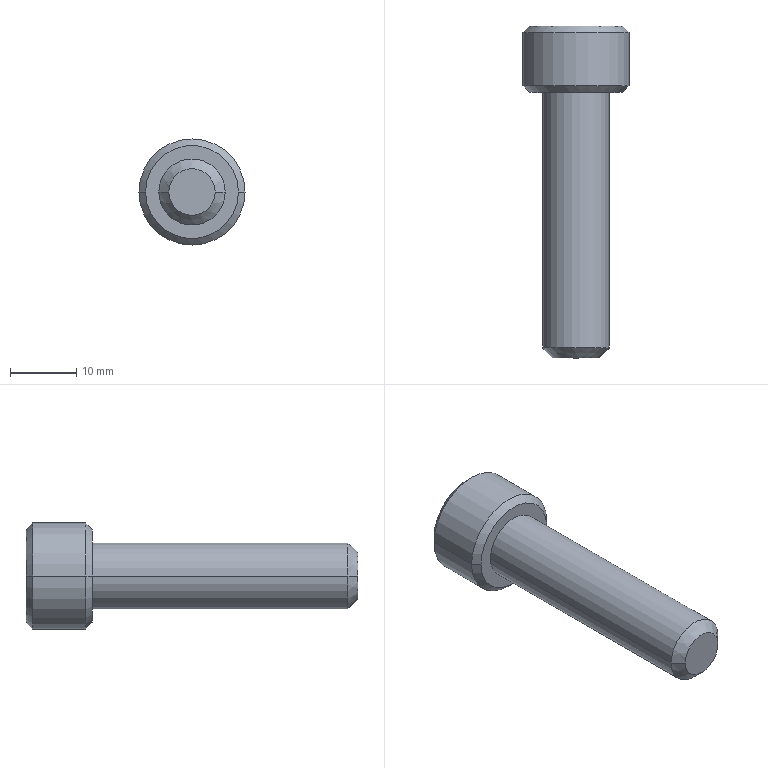Part | STEP file | BB62-M10-40L-1 | 1 solid | 27 faces | box 16 x 50 x 16 mm | volume 4742 mm3 | plane 15 | cone 8 | cylinder 4 | commonest cylinder face diameters 10 x2 16 x2
STEP:
#1=CARTESIAN_POINT('',(0.,2.359,0.));
#2=VERTEX_POINT('',#1);
#3=CARTESIAN_POINT('',(4.575,5.,0.));
#4=VERTEX_POINT('',#3);
#5=CARTESIAN_POINT('',(0.,2.359,0.));
#6=DIRECTION('',(0.866,0.5,0.));
#7=VECTOR('',#6,1000.);
#8=LINE('',#5,#7);
#9=EDGE_CURVE('',#2,#4,#8,.T.);
#10=ORIENTED_EDGE('',*,*,#9,.F.);
#11=CARTESIAN_POINT('',(-4.575,5.,0.));
#12=VERTEX_POINT('',#11);
#13=CARTESIAN_POINT('',(0.,2.359,0.));
#14=DIRECTION('',(-0.866,0.5,0.));
#15=VECTOR('',#14,1000.);
#16=LINE('',#13,#15);
#17=EDGE_CURVE('',#2,#12,#16,.T.);
#18=ORIENTED_EDGE('',*,*,#17,.T.);
#19=CARTESIAN_POINT('',(-3.962,5.,2.288));
#20=VERTEX_POINT('',#19);
#21=CARTESIAN_POINT('',(0.,5.,0.));
#22=DIRECTION('',(0.,-1.,0.));
#23=DIRECTION('',(-1.,0.,0.));
#24=AXIS2_PLACEMENT_3D('',#21,#22,#23);
#25=CIRCLE('',#24,4.575);
#26=EDGE_CURVE('',#20,#12,#25,.T.);
#27=ORIENTED_EDGE('',*,*,#26,.F.);
#28=CARTESIAN_POINT('',(0.,5.,4.575));
#29=VERTEX_POINT('',#28);
#30=CARTESIAN_POINT('',(0.,5.,0.));
#31=DIRECTION('',(0.,-1.,0.));
#32=DIRECTION('',(-1.,0.,0.));
#33=AXIS2_PLACEMENT_3D('',#30,#31,#32);
#34=CIRCLE('',#33,4.575);
#35=EDGE_CURVE('',#29,#20,#34,.T.);
#36=ORIENTED_EDGE('',*,*,#35,.F.);
#37=CARTESIAN_POINT('',(3.962,5.,2.287));
#38=VERTEX_POINT('',#37);
#39=CARTESIAN_POINT('',(0.,5.,0.));
#40=DIRECTION('',(0.,-1.,0.));
#41=DIRECTION('',(-1.,0.,0.));
#42=AXIS2_PLACEMENT_3D('',#39,#40,#41);
#43=CIRCLE('',#42,4.575);
#44=EDGE_CURVE('',#38,#29,#43,.T.);
#45=ORIENTED_EDGE('',*,*,#44,.F.);
#46=CARTESIAN_POINT('',(0.,5.,0.));
#47=DIRECTION('',(0.,-1.,0.));
#48=DIRECTION('',(-1.,0.,0.));
#49=AXIS2_PLACEMENT_3D('',#46,#47,#48);
#50=CIRCLE('',#49,4.575);
#51=EDGE_CURVE('',#4,#38,#50,.T.);
#52=ORIENTED_EDGE('',*,*,#51,.F.);
#53=EDGE_LOOP('',(#10,#18,#27,#36,#45,#52));
#54=FACE_OUTER_BOUND('',#53,.T.);
#55=CARTESIAN_POINT('',(0.,1002.359,0.));
#56=DIRECTION('',(0.,1.,0.));
#57=DIRECTION('',(1.,0.,0.));
#58=AXIS2_PLACEMENT_3D('',#55,#56,#57);
#59=CONICAL_SURFACE('',#58,1732.051,1.047);
#60=ADVANCED_FACE('',(#54),#59,.F.);
#61=CARTESIAN_POINT('',(3.5,-40.,0.));
#62=VERTEX_POINT('',#61);
#63=CARTESIAN_POINT('',(-3.5,-40.,0.));
#64=VERTEX_POINT('',#63);
#65=CARTESIAN_POINT('',(0.,-40.,0.));
#66=DIRECTION('',(0.,1.,0.));
#67=DIRECTION('',(1.,0.,0.));
#68=AXIS2_PLACEMENT_3D('',#65,#66,#67);
#69=CIRCLE('',#68,3.5);
#70=EDGE_CURVE('',#62,#64,#69,.T.);
#71=ORIENTED_EDGE('',*,*,#70,.T.);
#72=CARTESIAN_POINT('',(-5.,-38.5,0.));
#73=VERTEX_POINT('',#72);
#74=CARTESIAN_POINT('',(-3.5,-40.,0.));
#75=DIRECTION('',(-0.7071,0.7071,0.));
#76=VECTOR('',#75,1000.);
#77=LINE('',#74,#76);
#78=EDGE_CURVE('',#64,#73,#77,.T.);
#79=ORIENTED_EDGE('',*,*,#78,.T.);
#80=CARTESIAN_POINT('',(5.,-38.5,0.));
#81=VERTEX_POINT('',#80);
#82=CARTESIAN_POINT('',(0.,-38.5,0.));
#83=DIRECTION('',(0.,-1.,0.));
#84=DIRECTION('',(-1.,0.,0.));
#85=AXIS2_PLACEMENT_3D('',#82,#83,#84);
#86=CIRCLE('',#85,5.);
#87=EDGE_CURVE('',#73,#81,#86,.T.);
#88=ORIENTED_EDGE('',*,*,#87,.T.);
#89=CARTESIAN_POINT('',(3.5,-40.,0.));
#90=DIRECTION('',(0.7071,0.7071,0.));
#91=VECTOR('',#90,1000.);
#92=LINE('',#89,#91);
#93=EDGE_CURVE('',#62,#81,#92,.T.);
#94=ORIENTED_EDGE('',*,*,#93,.F.);
#95=EDGE_LOOP('',(#71,#79,#88,#94));
#96=FACE_OUTER_BOUND('',#95,.T.);
#97=CARTESIAN_POINT('',(0.,-40.,0.));
#98=DIRECTION('',(0.,1.,0.));
#99=DIRECTION('',(1.,0.,0.));
#100=AXIS2_PLACEMENT_3D('',#97,#98,#99);
#101=CONICAL_SURFACE('',#100,3.5,0.7854);
#102=ADVANCED_FACE('',(#96),#101,.T.);
#103=ORIENTED_EDGE('',*,*,#87,.F.);
#104=CARTESIAN_POINT('',(-5.,0.,0.));
#105=VERTEX_POINT('',#104);
#106=CARTESIAN_POINT('',(-5.,-38.5,0.));
#107=DIRECTION('',(0.,1.,0.));
#108=VECTOR('',#107,1000.);
#109=LINE('',#106,#108);
#110=EDGE_CURVE('',#73,#105,#109,.T.);
#111=ORIENTED_EDGE('',*,*,#110,.T.);
#112=CARTESIAN_POINT('',(5.,0.,0.));
#113=VERTEX_POINT('',#112);
#114=CARTESIAN_POINT('',(0.,0.,0.));
#115=DIRECTION('',(0.,-1.,0.));
#116=DIRECTION('',(-1.,0.,0.));
#117=AXIS2_PLACEMENT_3D('',#114,#115,#116);
#118=CIRCLE('',#117,5.);
#119=EDGE_CURVE('',#105,#113,#118,.T.);
#120=ORIENTED_EDGE('',*,*,#119,.T.);
#121=CARTESIAN_POINT('',(5.,-38.5,0.));
#122=DIRECTION('',(0.,1.,0.));
#123=VECTOR('',#122,1000.);
#124=LINE('',#121,#123);
#125=EDGE_CURVE('',#81,#113,#124,.T.);
#126=ORIENTED_EDGE('',*,*,#125,.F.);
#127=EDGE_LOOP('',(#103,#111,#120,#126));
#128=FACE_OUTER_BOUND('',#127,.T.);
#129=CARTESIAN_POINT('',(0.,-38.5,0.));
#130=DIRECTION('',(0.,1.,0.));
#131=DIRECTION('',(1.,0.,0.));
#132=AXIS2_PLACEMENT_3D('',#129,#130,#131);
#133=CYLINDRICAL_SURFACE('',#132,5.);
#134=ADVANCED_FACE('',(#128),#133,.T.);
#135=CARTESIAN_POINT('',(-7.,10.,0.));
#136=VERTEX_POINT('',#135);
#137=CARTESIAN_POINT('',(7.,10.,0.));
#138=VERTEX_POINT('',#137);
#139=CARTESIAN_POINT('',(0.,10.,0.));
#140=DIRECTION('',(0.,-1.,0.));
#141=DIRECTION('',(-1.,0.,0.));
#142=AXIS2_PLACEMENT_3D('',#139,#140,#141);
#143=CIRCLE('',#142,7.);
#144=EDGE_CURVE('',#136,#138,#143,.T.);
#145=ORIENTED_EDGE('',*,*,#144,.T.);
#146=CARTESIAN_POINT('',(8.,9.,0.));
#147=VERTEX_POINT('',#146);
#148=CARTESIAN_POINT('',(8.,9.,0.));
#149=DIRECTION('',(0.7071,-0.7071,0.));
#150=VECTOR('',#149,1000.);
#151=LINE('',#148,#150);
#152=EDGE_CURVE('',#138,#147,#151,.T.);
#153=ORIENTED_EDGE('',*,*,#152,.T.);
#154=CARTESIAN_POINT('',(-8.,9.,0.));
#155=VERTEX_POINT('',#154);
#156=CARTESIAN_POINT('',(0.,9.,0.));
#157=DIRECTION('',(0.,-1.,0.));
#158=DIRECTION('',(-1.,0.,0.));
#159=AXIS2_PLACEMENT_3D('',#156,#157,#158);
#160=CIRCLE('',#159,8.);
#161=EDGE_CURVE('',#155,#147,#160,.T.);
#162=ORIENTED_EDGE('',*,*,#161,.F.);
#163=CARTESIAN_POINT('',(-8.,9.,0.));
#164=DIRECTION('',(-0.7071,-0.7071,0.));
#165=VECTOR('',#164,1000.);
#166=LINE('',#163,#165);
#167=EDGE_CURVE('',#136,#155,#166,.T.);
#168=ORIENTED_EDGE('',*,*,#167,.F.);
#169=EDGE_LOOP('',(#145,#153,#162,#168));
#170=FACE_OUTER_BOUND('',#169,.T.);
#171=CARTESIAN_POINT('',(0.,9.,0.));
#172=DIRECTION('',(0.,-1.,0.));
#173=DIRECTION('',(-1.,0.,0.));
#174=AXIS2_PLACEMENT_3D('',#171,#172,#173);
#175=CONICAL_SURFACE('',#174,8.,0.7854);
#176=ADVANCED_FACE('',(#170),#175,.T.);
#177=ORIENTED_EDGE('',*,*,#161,.T.);
#178=CARTESIAN_POINT('',(8.,1.,0.));
#179=VERTEX_POINT('',#178);
#180=CARTESIAN_POINT('',(8.,1.62,0.));
#181=DIRECTION('',(0.,-1.,0.));
#182=VECTOR('',#181,1000.);
#183=LINE('',#180,#182);
#184=EDGE_CURVE('',#147,#179,#183,.T.);
#185=ORIENTED_EDGE('',*,*,#184,.T.);
#186=CARTESIAN_POINT('',(-8.,1.,0.));
#187=VERTEX_POINT('',#186);
#188=CARTESIAN_POINT('',(0.,1.,0.));
#189=DIRECTION('',(0.,-1.,0.));
#190=DIRECTION('',(-1.,0.,0.));
#191=AXIS2_PLACEMENT_3D('',#188,#189,#190);
#192=CIRCLE('',#191,8.);
#193=EDGE_CURVE('',#187,#179,#192,.T.);
#194=ORIENTED_EDGE('',*,*,#193,.F.);
#195=CARTESIAN_POINT('',(-8.,1.62,0.));
#196=DIRECTION('',(0.,-1.,0.));
#197=VECTOR('',#196,1000.);
#198=LINE('',#195,#197);
#199=EDGE_CURVE('',#155,#187,#198,.T.);
#200=ORIENTED_EDGE('',*,*,#199,.F.);
#201=EDGE_LOOP('',(#177,#185,#194,#200));
#202=FACE_OUTER_BOUND('',#201,.T.);
#203=CARTESIAN_POINT('',(0.,1.62,0.));
#204=DIRECTION('',(0.,-1.,0.));
#205=DIRECTION('',(-1.,0.,0.));
#206=AXIS2_PLACEMENT_3D('',#203,#204,#205);
#207=CYLINDRICAL_SURFACE('',#206,8.);
#208=ADVANCED_FACE('',(#202),#207,.T.);
#209=CARTESIAN_POINT('',(-7.,0.,0.));
#210=VERTEX_POINT('',#209);
#211=CARTESIAN_POINT('',(7.,0.,0.));
#212=VERTEX_POINT('',#211);
#213=CARTESIAN_POINT('',(0.,0.,0.));
#214=DIRECTION('',(0.,-1.,0.));
#215=DIRECTION('',(-1.,0.,0.));
#216=AXIS2_PLACEMENT_3D('',#213,#214,#215);
#217=CIRCLE('',#216,7.);
#218=EDGE_CURVE('',#210,#212,#217,.T.);
#219=ORIENTED_EDGE('',*,*,#218,.F.);
#220=CARTESIAN_POINT('',(-7.,0.,0.));
#221=DIRECTION('',(-0.7071,0.7071,0.));
#222=VECTOR('',#221,1000.);
#223=LINE('',#220,#222);
#224=EDGE_CURVE('',#210,#187,#223,.T.);
#225=ORIENTED_EDGE('',*,*,#224,.T.);
#226=ORIENTED_EDGE('',*,*,#193,.T.);
#227=CARTESIAN_POINT('',(7.,0.,0.));
#228=DIRECTION('',(0.7071,0.7071,0.));
#229=VECTOR('',#228,1000.);
#230=LINE('',#227,#229);
#231=EDGE_CURVE('',#212,#179,#230,.T.);
#232=ORIENTED_EDGE('',*,*,#231,.F.);
#233=EDGE_LOOP('',(#219,#225,#226,#232));
#234=FACE_OUTER_BOUND('',#233,.T.);
#235=CARTESIAN_POINT('',(0.,0.,0.));
#236=DIRECTION('',(0.,1.,0.));
#237=DIRECTION('',(1.,0.,0.));
#238=AXIS2_PLACEMENT_3D('',#235,#236,#237);
#239=CONICAL_SURFACE('',#238,7.,0.7854);
#240=ADVANCED_FACE('',(#234),#239,.T.);
#241=ORIENTED_EDGE('',*,*,#144,.F.);
#242=CARTESIAN_POINT('',(0.,10.,0.));
#243=DIRECTION('',(0.,-1.,0.));
#244=DIRECTION('',(-1.,0.,0.));
#245=AXIS2_PLACEMENT_3D('',#242,#243,#244);
#246=CIRCLE('',#245,7.);
#247=EDGE_CURVE('',#138,#136,#246,.T.);
#248=ORIENTED_EDGE('',*,*,#247,.F.);
#249=EDGE_LOOP('',(#241,#248));
#250=FACE_OUTER_BOUND('',#249,.T.);
#251=CARTESIAN_POINT('',(0.,10.,-4.575));
#252=VERTEX_POINT('',#251);
#253=CARTESIAN_POINT('',(-3.962,10.,-2.288));
#254=VERTEX_POINT('',#253);
#255=CARTESIAN_POINT('',(0.,10.,-4.575));
#256=DIRECTION('',(-0.866,0.,0.5));
#257=VECTOR('',#256,1000.);
#258=LINE('',#255,#257);
#259=EDGE_CURVE('',#252,#254,#258,.T.);
#260=ORIENTED_EDGE('',*,*,#259,.F.);
#261=CARTESIAN_POINT('',(3.962,10.,-2.288));
#262=VERTEX_POINT('',#261);
#263=CARTESIAN_POINT('',(3.962,10.,-2.288));
#264=DIRECTION('',(-0.866,0.,-0.5));
#265=VECTOR('',#264,1000.);
#266=LINE('',#263,#265);
#267=EDGE_CURVE('',#262,#252,#266,.T.);
#268=ORIENTED_EDGE('',*,*,#267,.F.);
#269=CARTESIAN_POINT('',(3.962,10.,2.287));
#270=VERTEX_POINT('',#269);
#271=CARTESIAN_POINT('',(3.962,10.,2.287));
#272=DIRECTION('',(0.,0.,-1.));
#273=VECTOR('',#272,1000.);
#274=LINE('',#271,#273);
#275=EDGE_CURVE('',#270,#262,#274,.T.);
#276=ORIENTED_EDGE('',*,*,#275,.F.);
#277=CARTESIAN_POINT('',(0.,10.,4.575));
#278=VERTEX_POINT('',#277);
#279=CARTESIAN_POINT('',(0.,10.,4.575));
#280=DIRECTION('',(0.866,0.,-0.5));
#281=VECTOR('',#280,1000.);
#282=LINE('',#279,#281);
#283=EDGE_CURVE('',#278,#270,#282,.T.);
#284=ORIENTED_EDGE('',*,*,#283,.F.);
#285=CARTESIAN_POINT('',(-3.962,10.,2.287));
#286=VERTEX_POINT('',#285);
#287=CARTESIAN_POINT('',(-3.962,10.,2.287));
#288=DIRECTION('',(0.866,0.,0.5));
#289=VECTOR('',#288,1000.);
#290=LINE('',#287,#289);
#291=EDGE_CURVE('',#286,#278,#290,.T.);
#292=ORIENTED_EDGE('',*,*,#291,.F.);
#293=CARTESIAN_POINT('',(-3.962,10.,-2.288));
#294=DIRECTION('',(0.,0.,1.));
#295=VECTOR('',#294,1000.);
#296=LINE('',#293,#295);
#297=EDGE_CURVE('',#254,#286,#296,.T.);
#298=ORIENTED_EDGE('',*,*,#297,.F.);
#299=EDGE_LOOP('',(#260,#268,#276,#284,#292,#298));
#300=FACE_BOUND('',#299,.T.);
#301=CARTESIAN_POINT('',(7.,10.,0.));
#302=DIRECTION('',(0.,1.,0.));
#303=DIRECTION('',(1.,0.,0.));
#304=AXIS2_PLACEMENT_3D('',#301,#302,#303);
#305=PLANE('',#304);
#306=ADVANCED_FACE('',(#250,#300),#305,.T.);
#307=CARTESIAN_POINT('',(0.,0.,0.));
#308=DIRECTION('',(0.,-1.,0.));
#309=DIRECTION('',(-1.,0.,0.));
#310=AXIS2_PLACEMENT_3D('',#307,#308,#309);
#311=CIRCLE('',#310,5.);
#312=EDGE_CURVE('',#113,#105,#311,.T.);
#313=ORIENTED_EDGE('',*,*,#312,.F.);
#314=ORIENTED_EDGE('',*,*,#119,.F.);
#315=EDGE_LOOP('',(#313,#314));
#316=FACE_BOUND('',#315,.T.);
#317=CARTESIAN_POINT('',(0.,0.,0.));
#318=DIRECTION('',(0.,-1.,0.));
#319=DIRECTION('',(-1.,0.,0.));
#320=AXIS2_PLACEMENT_3D('',#317,#318,#319);
#321=CIRCLE('',#320,7.);
#322=EDGE_CURVE('',#212,#210,#321,.T.);
#323=ORIENTED_EDGE('',*,*,#322,.T.);
#324=ORIENTED_EDGE('',*,*,#218,.T.);
#325=EDGE_LOOP('',(#323,#324));
#326=FACE_OUTER_BOUND('',#325,.T.);
#327=CARTESIAN_POINT('',(0.,0.,0.));
#328=DIRECTION('',(0.,-1.,0.));
#329=DIRECTION('',(-1.,0.,0.));
#330=AXIS2_PLACEMENT_3D('',#327,#328,#329);
#331=PLANE('',#330);
#332=ADVANCED_FACE('',(#316,#326),#331,.T.);
#333=ORIENTED_EDGE('',*,*,#224,.F.);
#334=ORIENTED_EDGE('',*,*,#322,.F.);
#335=ORIENTED_EDGE('',*,*,#231,.T.);
#336=CARTESIAN_POINT('',(0.,1.,0.));
#337=DIRECTION('',(0.,-1.,0.));
#338=DIRECTION('',(-1.,0.,0.));
#339=AXIS2_PLACEMENT_3D('',#336,#337,#338);
#340=CIRCLE('',#339,8.);
#341=EDGE_CURVE('',#179,#187,#340,.T.);
#342=ORIENTED_EDGE('',*,*,#341,.T.);
#343=EDGE_LOOP('',(#333,#334,#335,#342));
#344=FACE_OUTER_BOUND('',#343,.T.);
#345=CARTESIAN_POINT('',(0.,0.,0.));
#346=DIRECTION('',(0.,1.,0.));
#347=DIRECTION('',(1.,0.,0.));
#348=AXIS2_PLACEMENT_3D('',#345,#346,#347);
#349=CONICAL_SURFACE('',#348,7.,0.7854);
#350=ADVANCED_FACE('',(#344),#349,.T.);
#351=ORIENTED_EDGE('',*,*,#184,.F.);
#352=CARTESIAN_POINT('',(0.,9.,0.));
#353=DIRECTION('',(0.,-1.,0.));
#354=DIRECTION('',(-1.,0.,0.));
#355=AXIS2_PLACEMENT_3D('',#352,#353,#354);
#356=CIRCLE('',#355,8.);
#357=EDGE_CURVE('',#147,#155,#356,.T.);
#358=ORIENTED_EDGE('',*,*,#357,.T.);
#359=ORIENTED_EDGE('',*,*,#199,.T.);
#360=ORIENTED_EDGE('',*,*,#341,.F.);
#361=EDGE_LOOP('',(#351,#358,#359,#360));
#362=FACE_OUTER_BOUND('',#361,.T.);
#363=CARTESIAN_POINT('',(0.,1.62,0.));
#364=DIRECTION('',(0.,-1.,0.));
#365=DIRECTION('',(-1.,0.,0.));
#366=AXIS2_PLACEMENT_3D('',#363,#364,#365);
#367=CYLINDRICAL_SURFACE('',#366,8.);
#368=ADVANCED_FACE('',(#362),#367,.T.);
#369=ORIENTED_EDGE('',*,*,#152,.F.);
#370=ORIENTED_EDGE('',*,*,#247,.T.);
#371=ORIENTED_EDGE('',*,*,#167,.T.);
#372=ORIENTED_EDGE('',*,*,#357,.F.);
#373=EDGE_LOOP('',(#369,#370,#371,#372));
#374=FACE_OUTER_BOUND('',#373,.T.);
#375=CARTESIAN_POINT('',(0.,9.,0.));
#376=DIRECTION('',(0.,-1.,0.));
#377=DIRECTION('',(-1.,0.,0.));
#378=AXIS2_PLACEMENT_3D('',#375,#376,#377);
#379=CONICAL_SURFACE('',#378,8.,0.7854);
#380=ADVANCED_FACE('',(#374),#379,.T.);
#381=ORIENTED_EDGE('',*,*,#110,.F.);
#382=CARTESIAN_POINT('',(0.,-38.5,0.));
#383=DIRECTION('',(0.,-1.,0.));
#384=DIRECTION('',(-1.,0.,0.));
#385=AXIS2_PLACEMENT_3D('',#382,#383,#384);
#386=CIRCLE('',#385,5.);
#387=EDGE_CURVE('',#81,#73,#386,.T.);
#388=ORIENTED_EDGE('',*,*,#387,.F.);
#389=ORIENTED_EDGE('',*,*,#125,.T.);
#390=ORIENTED_EDGE('',*,*,#312,.T.);
#391=EDGE_LOOP('',(#381,#388,#389,#390));
#392=FACE_OUTER_BOUND('',#391,.T.);
#393=CARTESIAN_POINT('',(0.,-38.5,0.));
#394=DIRECTION('',(0.,1.,0.));
#395=DIRECTION('',(1.,0.,0.));
#396=AXIS2_PLACEMENT_3D('',#393,#394,#395);
#397=CYLINDRICAL_SURFACE('',#396,5.);
#398=ADVANCED_FACE('',(#392),#397,.T.);
#399=ORIENTED_EDGE('',*,*,#70,.F.);
#400=CARTESIAN_POINT('',(0.,-40.,0.));
#401=DIRECTION('',(0.,1.,0.));
#402=DIRECTION('',(1.,0.,0.));
#403=AXIS2_PLACEMENT_3D('',#400,#401,#402);
#404=CIRCLE('',#403,3.5);
#405=EDGE_CURVE('',#64,#62,#404,.T.);
#406=ORIENTED_EDGE('',*,*,#405,.F.);
#407=EDGE_LOOP('',(#399,#406));
#408=FACE_OUTER_BOUND('',#407,.T.);
#409=CARTESIAN_POINT('',(0.,-40.,0.));
#410=DIRECTION('',(0.,-1.,0.));
#411=DIRECTION('',(-1.,0.,0.));
#412=AXIS2_PLACEMENT_3D('',#409,#410,#411);
#413=PLANE('',#412);
#414=ADVANCED_FACE('',(#408),#413,.T.);
#415=ORIENTED_EDGE('',*,*,#78,.F.);
#416=ORIENTED_EDGE('',*,*,#405,.T.);
#417=ORIENTED_EDGE('',*,*,#93,.T.);
#418=ORIENTED_EDGE('',*,*,#387,.T.);
#419=EDGE_LOOP('',(#415,#416,#417,#418));
#420=FACE_OUTER_BOUND('',#419,.T.);
#421=CARTESIAN_POINT('',(0.,-40.,0.));
#422=DIRECTION('',(0.,1.,0.));
#423=DIRECTION('',(1.,0.,0.));
#424=AXIS2_PLACEMENT_3D('',#421,#422,#423);
#425=CONICAL_SURFACE('',#424,3.5,0.7854);
#426=ADVANCED_FACE('',(#420),#425,.T.);
#427=CARTESIAN_POINT('',(3.962,5.,-2.288));
#428=VERTEX_POINT('',#427);
#429=CARTESIAN_POINT('',(0.,5.,-4.575));
#430=VERTEX_POINT('',#429);
#431=CARTESIAN_POINT('',(3.962,5.,-2.288));
#432=DIRECTION('',(-0.866,0.,-0.5));
#433=VECTOR('',#432,1000.);
#434=LINE('',#431,#433);
#435=EDGE_CURVE('',#428,#430,#434,.T.);
#436=ORIENTED_EDGE('',*,*,#435,.F.);
#437=CARTESIAN_POINT('',(3.962,10.,-2.288));
#438=DIRECTION('',(0.,-1.,0.));
#439=VECTOR('',#438,1000.);
#440=LINE('',#437,#439);
#441=EDGE_CURVE('',#262,#428,#440,.T.);
#442=ORIENTED_EDGE('',*,*,#441,.F.);
#443=ORIENTED_EDGE('',*,*,#267,.T.);
#444=CARTESIAN_POINT('',(0.,10.,-4.575));
#445=DIRECTION('',(0.,-1.,0.));
#446=VECTOR('',#445,1000.);
#447=LINE('',#444,#446);
#448=EDGE_CURVE('',#252,#430,#447,.T.);
#449=ORIENTED_EDGE('',*,*,#448,.T.);
#450=EDGE_LOOP('',(#436,#442,#443,#449));
#451=FACE_OUTER_BOUND('',#450,.T.);
#452=CARTESIAN_POINT('',(3.962,10.,-2.288));
#453=DIRECTION('',(-0.5,0.,0.866));
#454=DIRECTION('',(0.866,0.,0.5));
#455=AXIS2_PLACEMENT_3D('',#452,#453,#454);
#456=PLANE('',#455);
#457=ADVANCED_FACE('',(#451),#456,.T.);
#458=CARTESIAN_POINT('',(-3.962,5.,-2.288));
#459=VERTEX_POINT('',#458);
#460=CARTESIAN_POINT('',(0.,5.,-4.575));
#461=DIRECTION('',(-0.866,0.,0.5));
#462=VECTOR('',#461,1000.);
#463=LINE('',#460,#462);
#464=EDGE_CURVE('',#430,#459,#463,.T.);
#465=ORIENTED_EDGE('',*,*,#464,.F.);
#466=ORIENTED_EDGE('',*,*,#448,.F.);
#467=ORIENTED_EDGE('',*,*,#259,.T.);
#468=CARTESIAN_POINT('',(-3.962,10.,-2.288));
#469=DIRECTION('',(0.,-1.,0.));
#470=VECTOR('',#469,1000.);
#471=LINE('',#468,#470);
#472=EDGE_CURVE('',#254,#459,#471,.T.);
#473=ORIENTED_EDGE('',*,*,#472,.T.);
#474=EDGE_LOOP('',(#465,#466,#467,#473));
#475=FACE_OUTER_BOUND('',#474,.T.);
#476=CARTESIAN_POINT('',(0.,10.,-4.575));
#477=DIRECTION('',(0.5,0.,0.866));
#478=DIRECTION('',(0.866,0.,-0.5));
#479=AXIS2_PLACEMENT_3D('',#476,#477,#478);
#480=PLANE('',#479);
#481=ADVANCED_FACE('',(#475),#480,.T.);
#482=CARTESIAN_POINT('',(-3.962,5.,-2.288));
#483=DIRECTION('',(0.,0.,1.));
#484=VECTOR('',#483,1000.);
#485=LINE('',#482,#484);
#486=EDGE_CURVE('',#459,#20,#485,.T.);
#487=ORIENTED_EDGE('',*,*,#486,.F.);
#488=ORIENTED_EDGE('',*,*,#472,.F.);
#489=ORIENTED_EDGE('',*,*,#297,.T.);
#490=CARTESIAN_POINT('',(-3.962,10.,2.287));
#491=DIRECTION('',(0.,-1.,0.));
#492=VECTOR('',#491,1000.);
#493=LINE('',#490,#492);
#494=EDGE_CURVE('',#286,#20,#493,.T.);
#495=ORIENTED_EDGE('',*,*,#494,.T.);
#496=EDGE_LOOP('',(#487,#488,#489,#495));
#497=FACE_OUTER_BOUND('',#496,.T.);
#498=CARTESIAN_POINT('',(-3.962,10.,-2.288));
#499=DIRECTION('',(1.,0.,0.));
#500=DIRECTION('',(0.,0.,-1.));
#501=AXIS2_PLACEMENT_3D('',#498,#499,#500);
#502=PLANE('',#501);
#503=ADVANCED_FACE('',(#497),#502,.T.);
#504=CARTESIAN_POINT('',(-3.962,5.,2.287));
#505=DIRECTION('',(0.866,0.,0.5));
#506=VECTOR('',#505,1000.);
#507=LINE('',#504,#506);
#508=EDGE_CURVE('',#20,#29,#507,.T.);
#509=ORIENTED_EDGE('',*,*,#508,.F.);
#510=ORIENTED_EDGE('',*,*,#494,.F.);
#511=ORIENTED_EDGE('',*,*,#291,.T.);
#512=CARTESIAN_POINT('',(0.,10.,4.575));
#513=DIRECTION('',(0.,-1.,0.));
#514=VECTOR('',#513,1000.);
#515=LINE('',#512,#514);
#516=EDGE_CURVE('',#278,#29,#515,.T.);
#517=ORIENTED_EDGE('',*,*,#516,.T.);
#518=EDGE_LOOP('',(#509,#510,#511,#517));
#519=FACE_OUTER_BOUND('',#518,.T.);
#520=CARTESIAN_POINT('',(-3.962,10.,2.287));
#521=DIRECTION('',(0.5,0.,-0.866));
#522=DIRECTION('',(-0.866,0.,-0.5));
#523=AXIS2_PLACEMENT_3D('',#520,#521,#522);
#524=PLANE('',#523);
#525=ADVANCED_FACE('',(#519),#524,.T.);
#526=CARTESIAN_POINT('',(0.,5.,4.575));
#527=DIRECTION('',(0.866,0.,-0.5));
#528=VECTOR('',#527,1000.);
#529=LINE('',#526,#528);
#530=EDGE_CURVE('',#29,#38,#529,.T.);
#531=ORIENTED_EDGE('',*,*,#530,.F.);
#532=ORIENTED_EDGE('',*,*,#516,.F.);
#533=ORIENTED_EDGE('',*,*,#283,.T.);
#534=CARTESIAN_POINT('',(3.962,10.,2.287));
#535=DIRECTION('',(0.,-1.,0.));
#536=VECTOR('',#535,1000.);
#537=LINE('',#534,#536);
#538=EDGE_CURVE('',#270,#38,#537,.T.);
#539=ORIENTED_EDGE('',*,*,#538,.T.);
#540=EDGE_LOOP('',(#531,#532,#533,#539));
#541=FACE_OUTER_BOUND('',#540,.T.);
#542=CARTESIAN_POINT('',(0.,10.,4.575));
#543=DIRECTION('',(-0.5,0.,-0.866));
#544=DIRECTION('',(-0.866,0.,0.5));
#545=AXIS2_PLACEMENT_3D('',#542,#543,#544);
#546=PLANE('',#545);
#547=ADVANCED_FACE('',(#541),#546,.T.);
#548=CARTESIAN_POINT('',(3.962,5.,2.287));
#549=DIRECTION('',(0.,0.,-1.));
#550=VECTOR('',#549,1000.);
#551=LINE('',#548,#550);
#552=EDGE_CURVE('',#38,#428,#551,.T.);
#553=ORIENTED_EDGE('',*,*,#552,.F.);
#554=ORIENTED_EDGE('',*,*,#538,.F.);
#555=ORIENTED_EDGE('',*,*,#275,.T.);
#556=ORIENTED_EDGE('',*,*,#441,.T.);
#557=EDGE_LOOP('',(#553,#554,#555,#556));
#558=FACE_OUTER_BOUND('',#557,.T.);
#559=CARTESIAN_POINT('',(3.962,10.,2.287));
#560=DIRECTION('',(-1.,0.,0.));
#561=DIRECTION('',(0.,0.,1.));
#562=AXIS2_PLACEMENT_3D('',#559,#560,#561);
#563=PLANE('',#562);
#564=ADVANCED_FACE('',(#558),#563,.T.);
#565=ORIENTED_EDGE('',*,*,#435,.T.);
#566=CARTESIAN_POINT('',(0.,5.,0.));
#567=DIRECTION('',(0.,-1.,0.));
#568=DIRECTION('',(-1.,0.,0.));
#569=AXIS2_PLACEMENT_3D('',#566,#567,#568);
#570=CIRCLE('',#569,4.575);
#571=EDGE_CURVE('',#430,#428,#570,.T.);
#572=ORIENTED_EDGE('',*,*,#571,.T.);
#573=EDGE_LOOP('',(#565,#572));
#574=FACE_OUTER_BOUND('',#573,.T.);
#575=CARTESIAN_POINT('',(0.,5.,0.));
#576=DIRECTION('',(0.,1.,0.));
#577=DIRECTION('',(1.,0.,0.));
#578=AXIS2_PLACEMENT_3D('',#575,#576,#577);
#579=PLANE('',#578);
#580=ADVANCED_FACE('',(#574),#579,.F.);
#581=ORIENTED_EDGE('',*,*,#552,.T.);
#582=CARTESIAN_POINT('',(0.,5.,0.));
#583=DIRECTION('',(0.,-1.,0.));
#584=DIRECTION('',(-1.,0.,0.));
#585=AXIS2_PLACEMENT_3D('',#582,#583,#584);
#586=CIRCLE('',#585,4.575);
#587=EDGE_CURVE('',#428,#4,#586,.T.);
#588=ORIENTED_EDGE('',*,*,#587,.T.);
#589=ORIENTED_EDGE('',*,*,#51,.T.);
#590=EDGE_LOOP('',(#581,#588,#589));
#591=FACE_OUTER_BOUND('',#590,.T.);
#592=CARTESIAN_POINT('',(0.,5.,0.));
#593=DIRECTION('',(0.,1.,0.));
#594=DIRECTION('',(1.,0.,0.));
#595=AXIS2_PLACEMENT_3D('',#592,#593,#594);
#596=PLANE('',#595);
#597=ADVANCED_FACE('',(#591),#596,.F.);
#598=ORIENTED_EDGE('',*,*,#530,.T.);
#599=ORIENTED_EDGE('',*,*,#44,.T.);
#600=EDGE_LOOP('',(#598,#599));
#601=FACE_OUTER_BOUND('',#600,.T.);
#602=CARTESIAN_POINT('',(0.,5.,0.));
#603=DIRECTION('',(0.,1.,0.));
#604=DIRECTION('',(1.,0.,0.));
#605=AXIS2_PLACEMENT_3D('',#602,#603,#604);
#606=PLANE('',#605);
#607=ADVANCED_FACE('',(#601),#606,.F.);
#608=ORIENTED_EDGE('',*,*,#508,.T.);
#609=ORIENTED_EDGE('',*,*,#35,.T.);
#610=EDGE_LOOP('',(#608,#609));
#611=FACE_OUTER_BOUND('',#610,.T.);
#612=CARTESIAN_POINT('',(0.,5.,0.));
#613=DIRECTION('',(0.,1.,0.));
#614=DIRECTION('',(1.,0.,0.));
#615=AXIS2_PLACEMENT_3D('',#612,#613,#614);
#616=PLANE('',#615);
#617=ADVANCED_FACE('',(#611),#616,.F.);
#618=ORIENTED_EDGE('',*,*,#486,.T.);
#619=ORIENTED_EDGE('',*,*,#26,.T.);
#620=CARTESIAN_POINT('',(0.,5.,0.));
#621=DIRECTION('',(0.,-1.,0.));
#622=DIRECTION('',(-1.,0.,0.));
#623=AXIS2_PLACEMENT_3D('',#620,#621,#622);
#624=CIRCLE('',#623,4.575);
#625=EDGE_CURVE('',#12,#459,#624,.T.);
#626=ORIENTED_EDGE('',*,*,#625,.T.);
#627=EDGE_LOOP('',(#618,#619,#626));
#628=FACE_OUTER_BOUND('',#627,.T.);
#629=CARTESIAN_POINT('',(0.,5.,0.));
#630=DIRECTION('',(0.,1.,0.));
#631=DIRECTION('',(1.,0.,0.));
#632=AXIS2_PLACEMENT_3D('',#629,#630,#631);
#633=PLANE('',#632);
#634=ADVANCED_FACE('',(#628),#633,.F.);
#635=ORIENTED_EDGE('',*,*,#464,.T.);
#636=CARTESIAN_POINT('',(0.,5.,0.));
#637=DIRECTION('',(0.,-1.,0.));
#638=DIRECTION('',(-1.,0.,0.));
#639=AXIS2_PLACEMENT_3D('',#636,#637,#638);
#640=CIRCLE('',#639,4.575);
#641=EDGE_CURVE('',#459,#430,#640,.T.);
#642=ORIENTED_EDGE('',*,*,#641,.T.);
#643=EDGE_LOOP('',(#635,#642));
#644=FACE_OUTER_BOUND('',#643,.T.);
#645=CARTESIAN_POINT('',(0.,5.,0.));
#646=DIRECTION('',(0.,1.,0.));
#647=DIRECTION('',(1.,0.,0.));
#648=AXIS2_PLACEMENT_3D('',#645,#646,#647);
#649=PLANE('',#648);
#650=ADVANCED_FACE('',(#644),#649,.F.);
#651=ORIENTED_EDGE('',*,*,#17,.F.);
#652=ORIENTED_EDGE('',*,*,#9,.T.);
#653=ORIENTED_EDGE('',*,*,#587,.F.);
#654=ORIENTED_EDGE('',*,*,#571,.F.);
#655=ORIENTED_EDGE('',*,*,#641,.F.);
#656=ORIENTED_EDGE('',*,*,#625,.F.);
#657=EDGE_LOOP('',(#651,#652,#653,#654,#655,#656));
#658=FACE_OUTER_BOUND('',#657,.T.);
#659=CARTESIAN_POINT('',(0.,1002.359,0.));
#660=DIRECTION('',(0.,1.,0.));
#661=DIRECTION('',(1.,0.,0.));
#662=AXIS2_PLACEMENT_3D('',#659,#660,#661);
#663=CONICAL_SURFACE('',#662,1732.051,1.047);
#664=ADVANCED_FACE('',(#658),#663,.F.);
#665=CLOSED_SHELL('',(#60,#102,#134,#176,#208,#240,#306,#332,#350,#368,#380,#398,#414,#426,#457,#481,#503,#525,#547,#564,#580,#597,#607,#617,#634,#650,#664));
#666=MANIFOLD_SOLID_BREP('',#665);
#667=CARTESIAN_POINT('',(0.,0.,0.));
#668=DIRECTION('',(0.,0.,1.));
#669=DIRECTION('',(1.,0.,0.));
#670=AXIS2_PLACEMENT_3D('',#667,#668,#669);
#671=(LENGTH_UNIT()NAMED_UNIT(*)SI_UNIT(.MILLI.,.METRE.));
#672=UNCERTAINTY_MEASURE_WITH_UNIT(LENGTH_MEASURE(0.00001),#671,'','');
#673=(NAMED_UNIT(*)PLANE_ANGLE_UNIT()SI_UNIT($,.RADIAN.));
#674=(NAMED_UNIT(*)SI_UNIT($,.STERADIAN.)SOLID_ANGLE_UNIT());
#675=(GEOMETRIC_REPRESENTATION_CONTEXT(3)GLOBAL_UNCERTAINTY_ASSIGNED_CONTEXT((#672))GLOBAL_UNIT_ASSIGNED_CONTEXT((#671,#673,#674))REPRESENTATION_CONTEXT('',''));
#676=ADVANCED_BREP_SHAPE_REPRESENTATION('',(#666,#670),#675);